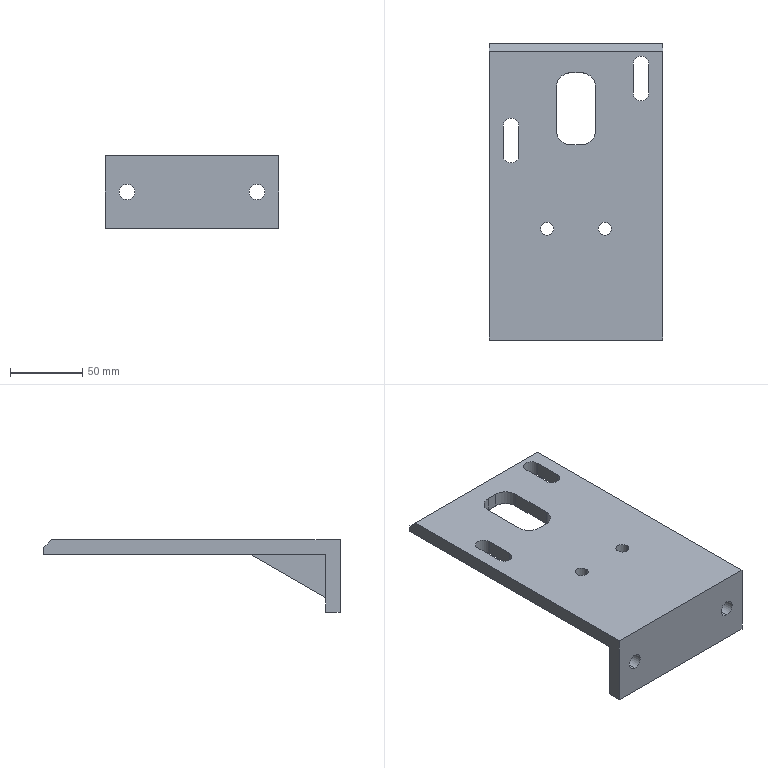NC program | NX | posted with a generic post | part box 120 x 205 x 50 mm
Lines 1 to 1489 of 11006:
N10 G17 G21 G94 G90
(FLOOR_WALL_1 , TOOL : D10)
N12 T15 M6
N14 G54
N16 G17 G0 G90 X12.169 Y-67. B0. C0. S9500 M3
N18 G43 Z30. H15
N20 Z0.003
N22 G94 G1 Z-0.998 F1000.
N24 X8.416 Y-60.5
N26 G3 X7.55 Y-60. R1.
N28 G1 X-87.4 F3500.
N30 Y60.
N32 X102.5
N34 Y-60.
N36 X7.55
N38 Y-55.
N40 X-82.4
N42 Y55.
N44 X97.5
N46 Y-55.
N48 X7.55
N50 Y-50.
N52 X-77.4
N54 Y50.
N56 X92.5
N58 Y-50.
N60 X7.55
N62 Y-45.
N64 X-72.4
N66 Y45.
N68 X87.5
N70 Y-45.
N72 X7.55
N74 Y-40.
N76 X-67.4
N78 Y40.
N80 X82.5
N82 Y-40.
N84 X7.55
N86 Y-35.
N88 X-62.4
N90 Y35.
N92 X77.5
N94 Y-35.
N96 X7.55
N98 Y-30.
N100 X-57.4
N102 Y30.
N104 X72.5
N106 Y-30.
N108 X7.55
N110 Y-25.
N112 X-52.4
N114 Y25.
N116 X67.5
N118 Y-25.
N120 X7.55
N122 Y-20.
N124 X-47.4
N126 Y20.
N128 X62.5
N130 Y-20.
N132 X7.55
N134 Y-15.
N136 X-42.4
N138 Y15.
N140 X57.5
N142 Y-15.
N144 X7.55
N146 Y-10.
N148 X-37.4
N150 Y10.
N152 X52.5
N154 Y-10.
N156 X7.55
N158 Y-5.
N160 X-32.4
N162 Y5.
N164 X47.5
N166 Y-5.
N168 X7.55
N170 Y0.
N172 X42.5
N174 X-27.4
N176 X7.55
N178 G3 X8.416 Y0.5 R1.
N180 G1 Z0.003
N182 G0 X12.169 Y-67. Z-0.995
N184 G1 Z-1.995 F1000.
N186 X8.416 Y-60.5
N188 G3 X7.55 Y-60. R1.
N190 G1 X-87.4 F3500.
N192 Y60.
N194 X102.5
N196 Y-60.
N198 X7.55
N200 Y-55.
N202 X-82.4
N204 Y55.
N206 X97.5
N208 Y-55.
N210 X7.55
N212 Y-50.
N214 X-77.4
N216 Y50.
N218 X92.5
N220 Y-50.
N222 X7.55
N224 Y-45.
N226 X-72.4
N228 Y45.
N230 X87.5
N232 Y-45.
N234 X7.55
N236 Y-40.
N238 X-67.4
N240 Y40.
N242 X82.5
N244 Y-40.
N246 X7.55
N248 Y-35.
N250 X-62.4
N252 Y35.
N254 X77.5
N256 Y-35.
N258 X7.55
N260 Y-30.
N262 X-57.4
N264 Y30.
N266 X72.5
N268 Y-30.
N270 X7.55
N272 Y-25.
N274 X-52.4
N276 Y25.
N278 X67.5
N280 Y-25.
N282 X7.55
N284 Y-20.
N286 X-47.4
N288 Y20.
N290 X62.5
N292 Y-20.
N294 X7.55
N296 Y-15.
N298 X-42.4
N300 Y15.
N302 X57.5
N304 Y-15.
N306 X7.55
N308 Y-10.
N310 X-37.4
N312 Y10.
N314 X52.5
N316 Y-10.
N318 X7.55
N320 Y-5.
N322 X-32.4
N324 Y5.
N326 X47.5
N328 Y-5.
N330 X7.55
N332 Y0.
N334 X42.5
N336 X-27.4
N338 X7.55
N340 G3 X8.416 Y0.5 R1.
N342 G1 Z-0.995
N344 G0 X12.169 Y-67. Z-1.993
N346 G1 Z-2.993 F1000.
N348 X8.416 Y-60.5
N350 G3 X7.55 Y-60. R1.
N352 G1 X-87.4 F3500.
N354 Y60.
N356 X102.5
N358 Y-60.
N360 X7.55
N362 Y-55.
N364 X-82.4
N366 Y55.
N368 X97.5
N370 Y-55.
N372 X7.55
N374 Y-50.
N376 X-77.4
N378 Y50.
N380 X92.5
N382 Y-50.
N384 X7.55
N386 Y-45.
N388 X-72.4
N390 Y45.
N392 X87.5
N394 Y-45.
N396 X7.55
N398 Y-40.
N400 X-67.4
N402 Y40.
N404 X82.5
N406 Y-40.
N408 X7.55
N410 Y-35.
N412 X-62.4
N414 Y35.
N416 X77.5
N418 Y-35.
N420 X7.55
N422 Y-30.
N424 X-57.4
N426 Y30.
N428 X72.5
N430 Y-30.
N432 X7.55
N434 Y-25.
N436 X-52.4
N438 Y25.
N440 X67.5
N442 Y-25.
N444 X7.55
N446 Y-20.
N448 X-47.4
N450 Y20.
N452 X62.5
N454 Y-20.
N456 X7.55
N458 Y-15.
N460 X-42.4
N462 Y15.
N464 X57.5
N466 Y-15.
N468 X7.55
N470 Y-10.
N472 X-37.4
N474 Y10.
N476 X52.5
N478 Y-10.
N480 X7.55
N482 Y-5.
N484 X-32.4
N486 Y5.
N488 X47.5
N490 Y-5.
N492 X7.55
N494 Y0.
N496 X42.5
N498 X-27.4
N500 X7.55
N502 G3 X8.416 Y0.5 R1.
N504 G1 Z-1.993
N506 G0 X12.169 Y-67. Z-2.99
N508 G1 Z-3.99 F1000.
N510 X8.416 Y-60.5
N512 G3 X7.55 Y-60. R1.
N514 G1 X-87.4 F3500.
N516 Y60.
N518 X102.5
N520 Y-60.
N522 X7.55
N524 Y-55.
N526 X-82.4
N528 Y55.
N530 X97.5
N532 Y-55.
N534 X7.55
N536 Y-50.
N538 X-77.4
N540 Y50.
N542 X92.5
N544 Y-50.
N546 X7.55
N548 Y-45.
N550 X-72.4
N552 Y45.
N554 X87.5
N556 Y-45.
N558 X7.55
N560 Y-40.
N562 X-67.4
N564 Y40.
N566 X82.5
N568 Y-40.
N570 X7.55
N572 Y-35.
N574 X-62.4
N576 Y35.
N578 X77.5
N580 Y-35.
N582 X7.55
N584 Y-30.
N586 X-57.4
N588 Y30.
N590 X72.5
N592 Y-30.
N594 X7.55
N596 Y-25.
N598 X-52.4
N600 Y25.
N602 X67.5
N604 Y-25.
N606 X7.55
N608 Y-20.
N610 X-47.4
N612 Y20.
N614 X62.5
N616 Y-20.
N618 X7.55
N620 Y-15.
N622 X-42.4
N624 Y15.
N626 X57.5
N628 Y-15.
N630 X7.55
N632 Y-10.
N634 X-37.4
N636 Y10.
N638 X52.5
N640 Y-10.
N642 X7.55
N644 Y-5.
N646 X-32.4
N648 Y5.
N650 X47.5
N652 Y-5.
N654 X7.55
N656 Y0.
N658 X42.5
N660 X-27.4
N662 X7.55
N664 G3 X8.416 Y0.5 R1.
N666 G1 Z-2.99
N668 G0 X12.169 Y-67. Z-3.988
N670 G1 Z-4.988 F1000.
N672 X8.416 Y-60.5
N674 G3 X7.55 Y-60. R1.
N676 G1 X-87.4 F3500.
N678 Y60.
N680 X102.5
N682 Y-60.
N684 X7.55
N686 Y-55.
N688 X-82.4
N690 Y55.
N692 X97.5
N694 Y-55.
N696 X7.55
N698 Y-50.
N700 X-77.4
N702 Y50.
N704 X92.5
N706 Y-50.
N708 X7.55
N710 Y-45.
N712 X-72.4
N714 Y45.
N716 X87.5
N718 Y-45.
N720 X7.55
N722 Y-40.
N724 X-67.4
N726 Y40.
N728 X82.5
N730 Y-40.
N732 X7.55
N734 Y-35.
N736 X-62.4
N738 Y35.
N740 X77.5
N742 Y-35.
N744 X7.55
N746 Y-30.
N748 X-57.4
N750 Y30.
N752 X72.5
N754 Y-30.
N756 X7.55
N758 Y-25.
N760 X-52.4
N762 Y25.
N764 X67.5
N766 Y-25.
N768 X7.55
N770 Y-20.
N772 X-47.4
N774 Y20.
N776 X62.5
N778 Y-20.
N780 X7.55
N782 Y-15.
N784 X-42.4
N786 Y15.
N788 X57.5
N790 Y-15.
N792 X7.55
N794 Y-10.
N796 X-37.4
N798 Y10.
N800 X52.5
N802 Y-10.
N804 X7.55
N806 Y-5.
N808 X-32.4
N810 Y5.
N812 X47.5
N814 Y-5.
N816 X7.55
N818 Y0.
N820 X42.5
N822 X-27.4
N824 X7.55
N826 G3 X8.416 Y0.5 R1.
N828 G1 Z-3.988
N830 G0 X12.169 Y-67. Z-4.985
N832 G1 Z-5.985 F1000.
N834 X8.416 Y-60.5
N836 G3 X7.55 Y-60. R1.
N838 G1 X-87.4 F3500.
N840 Y60.
N842 X102.5
N844 Y-60.
N846 X7.55
N848 Y-55.
N850 X-82.4
N852 Y55.
N854 X97.5
N856 Y-55.
N858 X7.55
N860 Y-50.
N862 X-77.4
N864 Y50.
N866 X92.5
N868 Y-50.
N870 X7.55
N872 Y-45.
N874 X-72.4
N876 Y45.
N878 X87.5
N880 Y-45.
N882 X7.55
N884 Y-40.
N886 X-67.4
N888 Y40.
N890 X82.5
N892 Y-40.
N894 X7.55
N896 Y-35.
N898 X-62.4
N900 Y35.
N902 X77.5
N904 Y-35.
N906 X7.55
N908 Y-30.
N910 X-57.4
N912 Y30.
N914 X72.5
N916 Y-30.
N918 X7.55
N920 Y-25.
N922 X-52.4
N924 Y25.
N926 X67.5
N928 Y-25.
N930 X7.55
N932 Y-20.
N934 X-47.4
N936 Y20.
N938 X62.5
N940 Y-20.
N942 X7.55
N944 Y-15.
N946 X-42.4
N948 Y15.
N950 X57.5
N952 Y-15.
N954 X7.55
N956 Y-10.
N958 X-37.4
N960 Y10.
N962 X52.5
N964 Y-10.
N966 X7.55
N968 Y-5.
N970 X-32.4
N972 Y5.
N974 X47.5
N976 Y-5.
N978 X7.55
N980 Y0.
N982 X42.5
N984 X-27.4
N986 X7.55
N988 G3 X8.416 Y0.5 R1.
N990 G1 Z-4.985
N992 G0 X12.169 Y-67. Z-5.983
N994 G1 Z-6.983 F1000.
N996 X8.416 Y-60.5
N998 G3 X7.55 Y-60. R1.
N1000 G1 X-87.4 F3500.
N1002 Y60.
N1004 X102.5
N1006 Y-60.
N1008 X7.55
N1010 Y-55.
N1012 X-82.4
N1014 Y55.
N1016 X97.5
N1018 Y-55.
N1020 X7.55
N1022 Y-50.
N1024 X-77.4
N1026 Y50.
N1028 X92.5
N1030 Y-50.
N1032 X7.55
N1034 Y-45.
N1036 X-72.4
N1038 Y45.
N1040 X87.5
N1042 Y-45.
N1044 X7.55
N1046 Y-40.
N1048 X-67.4
N1050 Y40.
N1052 X82.5
N1054 Y-40.
N1056 X7.55
N1058 Y-35.
N1060 X-62.4
N1062 Y35.
N1064 X77.5
N1066 Y-35.
N1068 X7.55
N1070 Y-30.
N1072 X-57.4
N1074 Y30.
N1076 X72.5
N1078 Y-30.
N1080 X7.55
N1082 Y-25.
N1084 X-52.4
N1086 Y25.
N1088 X67.5
N1090 Y-25.
N1092 X7.55
N1094 Y-20.
N1096 X-47.4
N1098 Y20.
N1100 X62.5
N1102 Y-20.
N1104 X7.55
N1106 Y-15.
N1108 X-42.4
N1110 Y15.
N1112 X57.5
N1114 Y-15.
N1116 X7.55
N1118 Y-10.
N1120 X-37.4
N1122 Y10.
N1124 X52.5
N1126 Y-10.
N1128 X7.55
N1130 Y-5.
N1132 X-32.4
N1134 Y5.
N1136 X47.5
N1138 Y-5.
N1140 X7.55
N1142 Y0.
N1144 X42.5
N1146 X-27.4
N1148 X7.55
N1150 G3 X8.416 Y0.5 R1.
N1152 G1 Z-5.983
N1154 G0 X12.169 Y-67. Z-6.98
N1156 G1 Z-7.98 F1000.
N1158 X8.416 Y-60.5
N1160 G3 X7.55 Y-60. R1.
N1162 G1 X-87.4 F3500.
N1164 Y60.
N1166 X102.5
N1168 Y-60.
N1170 X7.55
N1172 Y-55.
N1174 X-82.4
N1176 Y55.
N1178 X97.5
N1180 Y-55.
N1182 X7.55
N1184 Y-50.
N1186 X-77.4
N1188 Y50.
N1190 X92.5
N1192 Y-50.
N1194 X7.55
N1196 Y-45.
N1198 X-72.4
N1200 Y45.
N1202 X87.5
N1204 Y-45.
N1206 X7.55
N1208 Y-40.
N1210 X-67.4
N1212 Y40.
N1214 X82.5
N1216 Y-40.
N1218 X7.55
N1220 Y-35.
N1222 X-62.4
N1224 Y35.
N1226 X77.5
N1228 Y-35.
N1230 X7.55
N1232 Y-30.
N1234 X-57.4
N1236 Y30.
N1238 X72.5
N1240 Y-30.
N1242 X7.55
N1244 Y-25.
N1246 X-52.4
N1248 Y25.
N1250 X67.5
N1252 Y-25.
N1254 X7.55
N1256 Y-20.
N1258 X-47.4
N1260 Y20.
N1262 X62.5
N1264 Y-20.
N1266 X7.55
N1268 Y-15.
N1270 X-42.4
N1272 Y15.
N1274 X57.5
N1276 Y-15.
N1278 X7.55
N1280 Y-10.
N1282 X-37.4
N1284 Y10.
N1286 X52.5
N1288 Y-10.
N1290 X7.55
N1292 Y-5.
N1294 X-32.4
N1296 Y5.
N1298 X47.5
N1300 Y-5.
N1302 X7.55
N1304 Y0.
N1306 X42.5
N1308 X-27.4
N1310 X7.55
N1312 G3 X8.416 Y0.5 R1.
N1314 G1 Z-6.98
N1316 G0 X12.169 Y-67. Z-7.978
N1318 G1 Z-8.978 F1000.
N1320 X8.416 Y-60.5
N1322 G3 X7.55 Y-60. R1.
N1324 G1 X-87.4 F3500.
N1326 Y60.
N1328 X102.5
N1330 Y-60.
N1332 X7.55
N1334 Y-55.
N1336 X-82.4
N1338 Y55.
N1340 X97.5
N1342 Y-55.
N1344 X7.55
N1346 Y-50.
N1348 X-77.4
N1350 Y50.
N1352 X92.5
N1354 Y-50.
N1356 X7.55
N1358 Y-45.
N1360 X-72.4
N1362 Y45.
N1364 X87.5
N1366 Y-45.
N1368 X7.55
N1370 Y-40.
N1372 X-67.4
N1374 Y40.
N1376 X82.5
N1378 Y-40.
N1380 X7.55
N1382 Y-35.
N1384 X-62.4
N1386 Y35.
N1388 X77.5
N1390 Y-35.
N1392 X7.55
N1394 Y-30.
N1396 X-57.4
N1398 Y30.
N1400 X72.5
N1402 Y-30.
N1404 X7.55
N1406 Y-25.
N1408 X-52.4
N1410 Y25.
N1412 X67.5
N1414 Y-25.
N1416 X7.55
N1418 Y-20.
N1420 X-47.4
N1422 Y20.
N1424 X62.5
N1426 Y-20.
N1428 X7.55
N1430 Y-15.
N1432 X-42.4
N1434 Y15.
N1436 X57.5
N1438 Y-15.
N1440 X7.55
N1442 Y-10.
N1444 X-37.4
N1446 Y10.
N1448 X52.5
N1450 Y-10.
N1452 X7.55
N1454 Y-5.
N1456 X-32.4
N1458 Y5.
N1460 X47.5
N1462 Y-5.
N1464 X7.55
N1466 Y0.
N1468 X42.5
N1470 X-27.4
N1472 X7.55
N1474 G3 X8.416 Y0.5 R1.
N1476 G1 Z-7.978
N1478 G0 X12.169 Y-67. Z-8.975
N1480 G1 Z-9.975 F1000.
N1482 X8.416 Y-60.5
N1484 G3 X7.55 Y-60. R1.
N1486 G1 X-87.4 F3500.
N1488 Y60.
N1490 X102.5
N1492 Y-60.
N1494 X7.55
N1496 Y-55.
N1498 X-82.4
N1500 Y55.
N1502 X97.5
N1504 Y-55.
N1506 X7.55
N1508 Y-50.
N1510 X-77.4
N1512 Y50.
N1514 X92.5
N1516 Y-50.
N1518 X7.55
N1520 Y-45.
N1522 X-72.4
N1524 Y45.
N1526 X87.5
N1528 Y-45.
N1530 X7.55
N1532 Y-40.
N1534 X-67.4
N1536 Y40.
N1538 X82.5
N1540 Y-40.
N1542 X7.55
N1544 Y-35.
N1546 X-62.4
N1548 Y35.
N1550 X77.5
N1552 Y-35.
N1554 X7.55
N1556 Y-30.
N1558 X-57.4
N1560 Y30.
N1562 X72.5
N1564 Y-30.
N1566 X7.55
N1568 Y-25.
N1570 X-52.4
N1572 Y25.
N1574 X67.5
N1576 Y-25.
N1578 X7.55
N1580 Y-20.
N1582 X-47.4
N1584 Y20.
N1586 X62.5
N1588 Y-20.
N1590 X7.55
N1592 Y-15.
N1594 X-42.4
N1596 Y15.
N1598 X57.5
N1600 Y-15.
N1602 X7.55
N1604 Y-10.
N1606 X-37.4
N1608 Y10.
N1610 X52.5
N1612 Y-10.
N1614 X7.55
N1616 Y-5.
N1618 X-32.4
N1620 Y5.
N1622 X47.5
N1624 Y-5.
N1626 X7.55
N1628 Y0.
N1630 X42.5
N1632 X-27.4
N1634 X7.55
N1636 G3 X8.416 Y0.5 R1.
N1638 G1 Z-8.975
N1640 G0 X3.362 Y67. Z-9.973
N1642 G1 Z-10.973 F1000.
N1644 X7.115 Y60.5
N1646 G3 X7.981 Y60. R1.
N1648 G1 X102.5 F3500.
N1650 Y-60.
N1652 X-87.4
N1654 Y-30.1
N1656 X-85.716
N1658 Y-23.917
N1660 G3 X-85.111 Y-23.334 R0.6
N1662 G1 X-85.081 Y-15.959
N1664 G3 X-85.716 Y-15.363 R0.6
N1666 G1 Y-9.9
N1668 X-87.4
N1670 Y9.9
N1672 X-85.716
N1674 Y15.313
N1676 G3 X-85.111 Y15.897 R0.6
N1678 G1 X-85.081 Y23.271
N1680 G3 X-85.716 Y23.868 R0.6
N1682 G1 Y30.1
N1684 X-87.4
N1686 Y60.
N1688 X7.981
N1690 Y55.
N1692 X97.5
N1694 Y-55.
N1696 X-82.4
N1698 Y-33.843
N1700 G3 X-80.716 Y-30.1 R5.
N1702 G1 Y-25.849
N1704 G3 X-80.113 Y-23.475 R5.6
N1706 G1 X-80.076 Y-17.188
N1708 X-80.081 Y-15.94
N1710 G3 X-80.716 Y-13.371 R5.6
N1712 G1 Y-9.9
N1714 G3 X-82.4 Y-6.157 R5.
N1716 G1 Y6.157
N1718 G3 X-80.716 Y9.9 R5.
N1720 G1 Y13.382
N1722 G3 X-80.113 Y15.756 R5.6
N1724 G1 X-80.076 Y22.043
N1726 X-80.081 Y23.29
N1728 G3 X-80.716 Y25.859 R5.6
N1730 G1 Y30.1
N1732 G3 X-82.4 Y33.843 R5.
N1734 G1 Y55.
N1736 X7.981
N1738 Y50.
N1740 X92.5
N1742 Y-50.
N1744 X-77.4
N1746 Y-35.654
N1748 G3 X-75.716 Y-30.1 R10.
N1750 G1 Y-26.847
N1752 G3 X-75.115 Y-23.616 R10.6
N1754 G1 X-75.075 Y-22.221
N1756 X-75.081 Y-20.845
N1758 Y-15.922
N1760 G3 X-75.716 Y-12.348 R10.6
N1762 G1 Y-9.9
N1764 G3 X-77.4 Y-4.346 R10.
N1766 G1 Y4.346
N1768 G3 X-75.716 Y9.9 R10.
N1770 G1 Y12.383
N1772 G3 X-75.115 Y15.615 R10.6
N1774 G1 X-75.075 Y17.01
N1776 X-75.081 Y18.385
N1778 Y23.309
N1780 G3 X-75.716 Y26.883 R10.6
N1782 G1 Y30.1
N1784 G3 X-77.4 Y35.654 R10.
N1786 G1 Y50.
N1788 X7.981
N1790 Y45.
N1792 X87.5
N1794 Y-45.
N1796 X-72.4
N1798 Y-37.006
N1800 G3 X-70.716 Y-30.1 R15.
N1802 G1 Y-27.62
N1804 G3 X-70.117 Y-23.757 R15.6
N1806 G1 X-70.081 Y-15.903
N1808 G3 X-70.716 Y-11.556 R15.6
N1810 G1 Y-9.9
N1812 G3 X-72.4 Y-2.994 R15.
N1814 G1 Y2.994
N1816 G3 X-70.716 Y9.9 R15.
N1818 G1 Y11.611
N1820 G3 X-70.117 Y15.474 R15.6
N1822 G1 X-70.081 Y23.328
N1824 G3 X-70.716 Y27.675 R15.6
N1826 G1 Y30.1
N1828 G3 X-72.4 Y37.006 R15.
N1830 G1 Y45.
N1832 X7.981
N1834 Y40.
N1836 X82.5
N1838 Y-40.
N1840 X-67.4
N1842 Y-38.134
N1844 G3 X-65.716 Y-30.1 R20.
N1846 G1 Y-28.273
N1848 G3 X-65.117 Y-23.838 R20.6
N1850 G1 X-65.081 Y-15.905
N1852 G3 X-65.716 Y-10.886 R20.6
N1854 G1 Y-9.9
N1856 G3 X-67.4 Y-1.866 R20.
N1858 G1 Y1.866
N1860 G3 X-65.716 Y9.9 R20.
N1862 G1 Y10.957
N1864 G3 X-65.117 Y15.392 R20.6
N1866 G1 X-65.081 Y23.326
N1868 G3 X-65.716 Y28.345 R20.6
N1870 G1 Y30.1
N1872 G3 X-67.4 Y38.134 R20.
N1874 G1 Y40.
N1876 X7.981
N1878 Y35.
N1880 X77.5
N1882 Y-35.
N1884 X-61.2
N1886 G3 X-60.716 Y-30.1 R25.
N1888 G1 Y-28.85
N1890 G3 X-60.117 Y-23.913 R25.6
N1892 G1 X-60.081 Y-15.91
N1894 G3 X-60.716 Y-10.295 R25.6
N1896 G1 Y-9.9
N1898 G3 X-62.4 Y-0.879 R25.
N1900 G1 Y0.879
N1902 G3 X-60.716 Y9.9 R25.
N1904 G1 Y10.38
N1906 G3 X-60.117 Y15.318 R25.6
N1908 G1 X-60.081 Y23.321
N1910 G3 X-60.716 Y28.936 R25.6
N1912 G1 Y30.1
N1914 G3 X-61.2 Y35. R25.
N1916 G1 X7.981
N1918 Y30.
N1920 X72.5
N1922 Y-30.
N1924 X-55.716
N1926 Y-29.373
N1928 G3 X-55.118 Y-23.983 R30.6
N1930 G1 X-55.081 Y-15.916
N1932 G3 X-55.716 Y-9.758 R30.6
N1934 X-57.396 Y0. R30.
N1936 X-55.716 Y9.858 R30.
N1938 X-55.118 Y15.248 R30.6
N1940 G1 X-55.081 Y23.315
N1942 G3 X-55.716 Y29.471 R30.6
N1944 G1 Y30.
N1946 X7.981
N1948 Y25.
N1950 X67.5
N1952 Y-25.
N1954 X-50.15
N1956 G3 X-50.118 Y-24.049 R35.6
N1958 G1 X-50.081 Y-15.924
N1960 G3 X-50.722 Y-9.235 R35.6
N1962 X-52.145 Y0. R35.
N1964 X-50.72 Y9.355 R35.
N1966 X-50.118 Y15.182 R35.6
N1968 G1 X-50.081 Y23.307
N1970 G3 X-50.123 Y25. R35.6
N1972 G1 X7.981
N1974 Y20.
N1976 X62.5
N1978 Y-20.
N1980 X-45.099
N1982 X-45.081 Y-15.932
N1984 G3 X-45.733 Y-8.711 R40.6
N1986 X-46.96 Y0. R40.
N1988 X-45.729 Y8.852 R40.
N1990 X-45.119 Y15.078 R40.6
N1992 G1 X-45.096 Y20.
N1994 X7.981
N1996 Y15.
N1998 X57.5
N2000 Y-15.
N2002 X-40.091
N2004 G3 X-40.748 Y-8.187 R45.6
N2006 X-41.818 Y0. R45.
N2008 X-40.742 Y8.349 R45.
N2010 X-40.423 Y10.584 R45.6
N2012 X-40.119 Y15. R45.6
N2014 G1 X7.981
N2016 Y10.
N2018 X52.5
N2020 Y-10.
N2022 X-35.433
N2024 G3 X-35.766 Y-7.663 R50.6
N2026 X-36.705 Y0. R50.
N2028 X-35.758 Y7.845 R50.
N2030 X-35.457 Y10. R50.6
N2032 G1 X7.981
N2034 Y5.
N2036 X47.5
N2038 Y-5.
N2040 X-30.934
N2042 G3 X-31.614 Y0. R55.
N2044 X-30.934 Y5. R55.
N2046 G1 X7.981
N2048 Y0.
N2050 X42.5
N2052 X-26.538
N2054 X7.981
N2056 G3 X8.847 Y0.5 R1.
N2058 G1 Z-9.973
N2060 G0 X4.226 Y67. Z-10.97
N2062 G1 Z-11.97 F1000.
N2064 X7.979 Y60.5
N2066 G3 X8.845 Y60. R1.
N2068 G1 X102.5 F3500.
N2070 Y-60.
N2072 X-87.4
N2074 Y-30.1
N2076 X-83.988
N2078 Y-23.917
N2080 G3 X-83.39 Y-23.338 R0.6
N2082 G1 X-83.348 Y-22.099
N2084 X-83.36 Y-20.863
N2086 Y-15.956
N2088 G3 X-83.988 Y-15.362 R0.6
N2090 G1 Y-13.385
N2092 Y-9.9
N2094 X-87.4
N2096 Y9.9
N2098 X-83.988
N2100 Y15.313
N2102 G3 X-83.39 Y15.893 R0.6
N2104 G1 X-83.348 Y17.132
N2106 X-83.36 Y18.368
N2108 Y23.275
N2110 G3 X-83.988 Y23.869 R0.6
N2112 G1 Y25.846
N2114 Y30.1
N2116 X-87.4
N2118 Y60.
N2120 X8.845
N2122 Y55.
N2124 X97.5
N2126 Y-55.
N2128 X-82.4
N2130 Y-34.841
N2132 G3 X-78.988 Y-30.1 R5.
N2134 G1 Y-25.835
N2136 G3 X-78.393 Y-23.507 R5.6
N2138 G1 X-78.36 Y-15.909
N2140 G3 X-78.988 Y-13.385 R5.6
N2142 G1 Y-9.9
N2144 G3 X-82.4 Y-5.159 R5.
N2146 G1 Y5.159
N2148 G3 X-78.988 Y9.9 R5.
N2150 G1 Y13.395
N2152 G3 X-78.393 Y15.724 R5.6
N2154 G1 X-78.347 Y17.071
N2156 X-78.36 Y18.392
N2158 Y23.322
N2160 G3 X-78.988 Y25.846 R5.6
N2162 G1 Y30.1
N2164 G3 X-82.4 Y34.841 R5.
N2166 G1 Y55.
N2168 X8.845
N2170 Y50.
N2172 X92.5
N2174 Y-50.
N2176 X-77.4
N2178 Y-37.623
N2180 G3 X-73.988 Y-30.1 R10.
N2182 G1 Y-26.827
N2184 G3 X-73.393 Y-23.602 R10.6
N2186 G1 X-73.36 Y-15.896
N2188 G3 X-73.988 Y-12.367 R10.6
N2190 G1 Y-9.9
N2192 G3 X-77.4 Y-2.377 R10.
N2194 G1 Y2.377
N2196 G3 X-73.988 Y9.9 R10.
N2198 G1 Y12.403
N2200 G3 X-73.396 Y15.555 R10.6
N2202 G1 X-73.347 Y17.01
N2204 X-73.36 Y23.369
N2206 G3 X-73.988 Y26.863 R10.6
N2208 G1 Y30.1
N2210 G3 X-77.4 Y37.623 R10.
N2212 G1 Y50.
N2214 X8.845
N2216 Y45.
N2218 X87.5
N2220 Y-45.
N2222 X-72.4
N2224 Y-39.625
N2226 G3 X-68.988 Y-30.1 R15.
N2228 G1 Y-27.595
N2230 G3 X-68.394 Y-23.68 R15.6
N2232 G1 X-68.36 Y-15.892
N2234 G3 X-68.988 Y-11.58 R15.6
N2236 G1 Y-9.9
N2238 G3 X-72.4 Y-0.375 R15.
N2240 G1 Y0.375
N2242 G3 X-68.988 Y9.9 R15.
N2244 G1 Y11.635
N2246 G3 X-68.399 Y15.386 R15.6
N2248 G1 X-68.346 Y16.949
N2250 X-68.361 Y23.416
N2252 G3 X-68.988 Y27.651 R15.6
N2254 G1 Y30.1
N2256 G3 X-72.4 Y39.625 R15.
N2258 G1 Y45.
N2260 X8.845
N2262 Y40.
N2264 X82.5
N2266 Y-40.
N2268 X-66.61
N2270 G3 X-63.988 Y-30.1 R20.
N2272 G1 Y-28.245
N2274 G3 X-63.394 Y-23.749 R20.6
N2276 G1 X-63.36 Y-15.891
N2278 G3 X-63.988 Y-10.914 R20.6
N2280 G1 Y-9.9
N2282 G3 X-66.61 Y0. R20.
N2284 X-63.988 Y9.9 R20.
N2286 G1 Y10.986
N2288 G3 X-63.402 Y15.217 R20.6
N2290 G1 X-63.345 Y16.888
N2292 X-63.361 Y23.463
N2294 G3 X-63.988 Y28.317 R20.6
N2296 G1 Y30.1
N2298 G3 X-66.61 Y40. R20.
N2300 G1 X8.845
N2302 Y35.
N2304 X77.5
N2306 Y-35.
N2308 X-59.473
N2310 G3 X-58.988 Y-30.1 R25.
N2312 G1 Y-28.819
N2314 G3 X-58.394 Y-23.813 R25.6
N2316 G1 X-58.36 Y-15.893
N2318 G3 X-58.988 Y-10.326 R25.6
N2320 G1 Y-9.811
N2322 G3 X-61.032 Y0. R25.
N2324 X-58.988 Y9.9 R25.
N2326 G1 Y10.412
N2328 G3 X-58.404 Y15.048 R25.6
N2330 G1 X-58.344 Y16.827
N2332 X-58.361 Y23.51
N2334 G3 X-58.988 Y28.905 R25.6
N2336 G1 Y30.1
N2338 G3 X-59.473 Y35. R25.
N2340 G1 X8.845
N2342 Y30.
N2344 X72.5
N2346 Y-30.
N2348 X-53.988
N2350 Y-29.338
N2352 G3 X-53.394 Y-23.872 R30.6
N2354 G1 X-53.36 Y-15.897
N2356 G3 X-53.988 Y-9.793 R30.6
N2358 X-55.668 Y0. R30.
N2360 X-53.988 Y9.893 R30.
N2362 X-53.407 Y14.879 R30.6
N2364 G1 X-53.343 Y16.766
N2366 X-53.361 Y23.557
N2368 G3 X-53.988 Y29.437 R30.6
N2370 G1 Y30.
N2372 X8.845
N2374 Y25.
N2376 X67.5
N2378 Y-25.
N2380 X-48.429
N2382 G3 X-48.395 Y-23.928 R35.6
N2384 G1 X-48.36 Y-15.903
N2386 G3 X-48.993 Y-9.275 R35.6
N2388 X-50.417 Y0. R35.
N2390 X-48.991 Y9.396 R35.
N2392 X-48.41 Y14.71 R35.6
N2394 G1 X-48.361 Y23.604
N2396 G3 X-48.402 Y25. R35.6
N2398 G1 X8.845
N2400 Y20.
N2402 X62.5
N2404 Y-20.
N2406 X-43.378
N2408 X-43.36 Y-15.91
N2410 G3 X-44.004 Y-8.757 R40.6
N2412 X-45.232 Y0. R40.
N2414 X-44. Y8.899 R40.
N2416 X-43.411 Y14.612 R40.6
N2418 G1 X-43.381 Y20.
N2420 X8.845
N2422 Y15.
N2424 X57.5
N2426 Y-15.
N2428 X-38.37
N2430 G3 X-39.019 Y-8.239 R45.6
N2432 X-40.09 Y0. R45.
N2434 X-39.013 Y8.402 R45.
N2436 X-38.411 Y14.518 R45.6
N2438 G1 X-38.408 Y15.
N2440 X8.845
N2442 Y10.
N2444 X52.5
N2446 Y-10.
N2448 X-33.712
N2450 G3 X-34.035 Y-7.721 R50.6
N2452 X-34.978 Y0. R50.
N2454 X-34.028 Y7.904 R50.
N2456 X-33.737 Y10. R50.6
N2458 G1 X8.845
N2460 Y5.
N2462 X47.5
N2464 Y-5.
N2466 X-29.207
N2468 G3 X-29.886 Y0. R55.
N2470 X-29.207 Y5. R55.
N2472 G1 X8.845
N2474 Y0.
N2476 X42.5
N2478 X-24.81
N2480 X8.845
N2482 G3 X9.711 Y0.5 R1.
N2484 G1 Z-10.97
N2486 G0 X5.09 Y67. Z-11.968
N2488 G1 Z-12.968 F1000.
N2490 X8.843 Y60.5
N2492 G3 X9.709 Y60. R1.
N2494 G1 X102.5 F3500.
N2496 Y-60.
N2498 X-87.4
N2500 Y-30.1
N2502 X-82.26
N2504 Y-23.917
N2506 G3 X-81.654 Y-23.334 R0.6
N2508 G1 X-81.621 Y-17.186
N2510 X-81.639 Y-15.953
N2512 G3 X-82.26 Y-15.362 R0.6
N2514 G1 Y-9.9
N2516 X-87.4
N2518 Y9.9
N2520 X-82.26
N2522 Y15.313
N2524 G3 X-81.654 Y15.897 R0.6
N2526 G1 X-81.621 Y22.045
N2528 X-81.639 Y23.278
N2530 G3 X-82.26 Y23.869 R0.6
N2532 G1 Y30.1
N2534 X-87.4
N2536 Y60.
N2538 X9.709
N2540 Y55.
N2542 X97.5
N2544 Y-55.
N2546 X-82.4
N2548 Y-35.1
N2550 G3 X-77.26 Y-30.1 R5.
N2552 G1 Y-25.851
N2554 G3 X-76.656 Y-23.47 R5.6
N2556 G1 X-76.62 Y-22.14
N2558 X-76.633 Y-20.837
N2560 X-76.64 Y-15.877
N2562 G3 X-77.26 Y-13.399 R5.6
N2564 G1 Y-9.9
N2566 G3 X-82.26 Y-4.9 R5.
N2568 G1 X-82.4
N2570 Y4.9
N2572 G3 X-77.26 Y9.9 R5.
N2574 G1 Y13.38
N2576 G3 X-76.656 Y15.761 R5.6
N2578 G1 X-76.62 Y17.091
N2580 X-76.633 Y18.394
N2582 X-76.64 Y23.354
N2584 G3 X-77.26 Y25.832 R5.6
N2586 G1 Y30.1
N2588 G3 X-82.26 Y35.1 R5.
N2590 G1 X-82.4
N2592 Y55.
N2594 X9.709
N2596 Y50.
N2598 X92.5
N2600 Y-50.
N2602 X-77.4
N2604 Y-38.841
N2606 G3 X-72.26 Y-30.099 R10.
N2608 G1 Y-26.85
N2610 G3 X-71.658 Y-23.606 R10.6
N2612 G1 X-71.619 Y-22.183
N2614 X-71.633 Y-20.812
N2616 X-71.64 Y-15.802
N2618 G3 X-72.26 Y-12.387 R10.6
N2620 G1 Y-9.9
N2622 G3 X-77.4 Y-1.16 R10.
N2624 G1 Y1.159
N2626 G3 X-72.26 Y9.901 R10.
N2628 G1 Y12.381
N2630 G3 X-71.658 Y15.625 R10.6
N2632 G1 X-71.619 Y17.048
N2634 X-71.633 Y18.419
N2636 X-71.64 Y23.429
N2638 G3 X-72.26 Y26.844 R10.6
N2640 G1 Y30.1
N2642 G3 X-77.4 Y38.84 R10.
N2644 G1 Y50.
N2646 X9.709
N2648 Y45.
N2650 X87.5
N2652 Y-45.
N2654 X-72.4
N2656 Y-41.406
N2658 G3 X-67.26 Y-30.098 R15.
N2660 G1 Y-27.623
N2662 G3 X-66.66 Y-23.742 R15.6
N2664 G1 X-66.641 Y-15.727
N2666 G3 X-67.26 Y-11.604 R15.6
N2668 G1 Y-9.9
N2670 G3 X-70.99 Y-0.001 R15.
N2672 X-67.26 Y9.902 R15.
N2674 G1 Y11.608
N2676 G3 X-66.66 Y15.488 R15.6
N2678 G1 X-66.619 Y17.005
N2680 X-66.633 Y18.444
N2682 X-66.641 Y23.504
N2684 G3 X-67.26 Y27.627 R15.6
N2686 G1 Y30.1
N2688 G3 X-72.4 Y41.404 R15.
N2690 G1 Y45.
N2692 X9.709
N2694 Y40.
N2696 X82.5
N2698 Y-40.
N2700 X-64.881
N2702 G3 X-62.26 Y-30.097 R20.
N2704 G1 Y-28.277
N2706 G3 X-61.66 Y-23.817 R20.6
N2708 G1 X-61.641 Y-15.695
N2710 G3 X-62.26 Y-10.942 R20.6
N2712 G1 Y-9.9
N2714 G3 X-64.882 Y-0.001 R20.
N2716 X-62.26 Y9.903 R20.
N2718 G1 Y10.954
N2720 G3 X-61.662 Y15.352 R20.6
N2722 G1 X-61.618 Y16.962
N2724 X-61.633 Y18.469
N2726 X-61.642 Y23.579
N2728 G3 X-62.26 Y28.289 R20.6
N2730 G1 Y30.1
N2732 G3 X-64.882 Y40. R20.
N2734 G1 X9.709
N2736 Y35.
N2738 X77.5
N2740 Y-35.
N2742 X-57.745
N2744 G3 X-57.26 Y-30.096 R25.
N2746 G1 Y-28.854
N2748 G3 X-56.66 Y-23.883 R25.6
N2750 G1 X-56.641 Y-15.668
N2752 G3 X-57.26 Y-10.357 R25.6
N2754 G1 Y-9.84
N2756 G3 X-59.303 Y-0.001 R25.
N2758 X-57.26 Y9.904 R25.
N2760 G1 Y10.376
N2762 G3 X-56.664 Y15.216 R25.6
N2764 G1 X-56.642 Y23.655
N2766 G3 X-57.26 Y28.873 R25.6
N2768 G1 Y30.1
N2770 G3 X-57.745 Y35. R25.
N2772 G1 X9.709
N2774 Y30.
N2776 X72.5
N2778 Y-30.
N2780 X-52.26
N2782 Y-29.377
N2784 G3 X-51.66 Y-23.944 R30.6
N2786 G1 X-51.641 Y-15.646
N2788 G3 X-52.26 Y-9.828 R30.6
N2790 X-53.94 Y-0.001 R30.
N2792 X-52.26 Y9.854 R30.
N2794 X-51.664 Y15.141 R30.6
N2796 G1 X-51.642 Y23.686
N2798 G3 X-52.26 Y29.402 R30.6
N2800 G1 Y30.
N2802 X9.709
N2804 Y25.
N2806 X67.5
N2808 Y-25.
N2810 X-46.694
N2812 G3 X-46.661 Y-24.002 R35.6
N2814 G1 X-46.641 Y-15.626
N2816 G3 X-47.265 Y-9.316 R35.6
N2818 X-48.689 Y-0.001 R35.
N2820 X-47.264 Y9.35 R35.
N2822 X-46.664 Y15.072 R35.6
N2824 G1 X-46.642 Y23.754
N2826 G3 X-46.681 Y25. R35.6
N2828 G1 X9.709
N2830 Y20.
N2832 X62.5
N2834 Y-20.
N2836 X-41.651
N2838 X-41.641 Y-15.608
N2840 G3 X-42.275 Y-8.804 R40.6
N2842 X-43.504 Y-0.001 R40.
N2844 X-42.274 Y8.846 R40.
N2846 X-41.664 Y15.006 R40.6
N2848 G1 X-41.652 Y20.
N2850 X9.709
N2852 Y15.
N2854 X57.5
N2856 Y-15.
N2858 X-36.649
N2860 G3 X-37.289 Y-8.291 R45.6
N2862 X-38.362 Y-0.001 R45.
N2864 X-37.287 Y8.343 R45.
N2866 X-36.967 Y10.584 R45.6
N2868 X-36.664 Y15. R45.6
N2870 G1 X9.709
N2872 Y10.
N2874 X52.5
N2876 Y-10.
N2878 X-31.992
N2880 G3 X-32.305 Y-7.779 R50.6
N2882 X-33.25 Y-0.001 R50.
N2884 X-32.303 Y7.839 R50.
N2886 X-32.001 Y10. R50.6
N2888 G1 X9.709
N2890 Y5.
N2892 X47.5
N2894 Y-5.
N2896 X-27.479
N2898 G3 X-28.158 Y-0.001 R55.
N2900 X-27.479 Y5. R55.
N2902 G1 X9.709
N2904 Y0.
N2906 X42.5
N2908 X-23.082
N2910 X9.709
N2912 G3 X10.575 Y0.5 R1.
N2914 G1 Z-11.968
N2916 G0 X5.954 Y67. Z-12.965
N2918 G1 Z-13.965 F1000.
N2920 X9.707 Y60.5
N2922 G3 X10.573 Y60. R1.
N2924 G1 X102.5 F3500.
N2926 Y-60.
N2928 X-87.4
N2930 Y-30.1
N2932 X-80.532
N2934 Y-23.917
N2936 X-80.489
N2938 G3 X-79.889 Y-23.315 R0.6
N2940 G1 Y-15.964
N2942 G3 X-79.958 Y-15.682 R0.6
N2944 X-80.532 Y-15.362 R0.602
N2946 G1 Y-9.9
N2948 X-87.4
N2950 Y9.9
N2952 X-80.532
N2954 Y15.313
N2956 X-80.489
N2958 G3 X-79.889 Y15.915 R0.6
N2960 G1 Y23.267
N2962 G3 X-79.958 Y23.549 R0.6
N2964 X-80.532 Y23.869 R0.602
N2966 G1 Y30.1
N2968 X-87.4
N2970 Y60.
N2972 X10.573
N2974 Y55.
N2976 X97.5